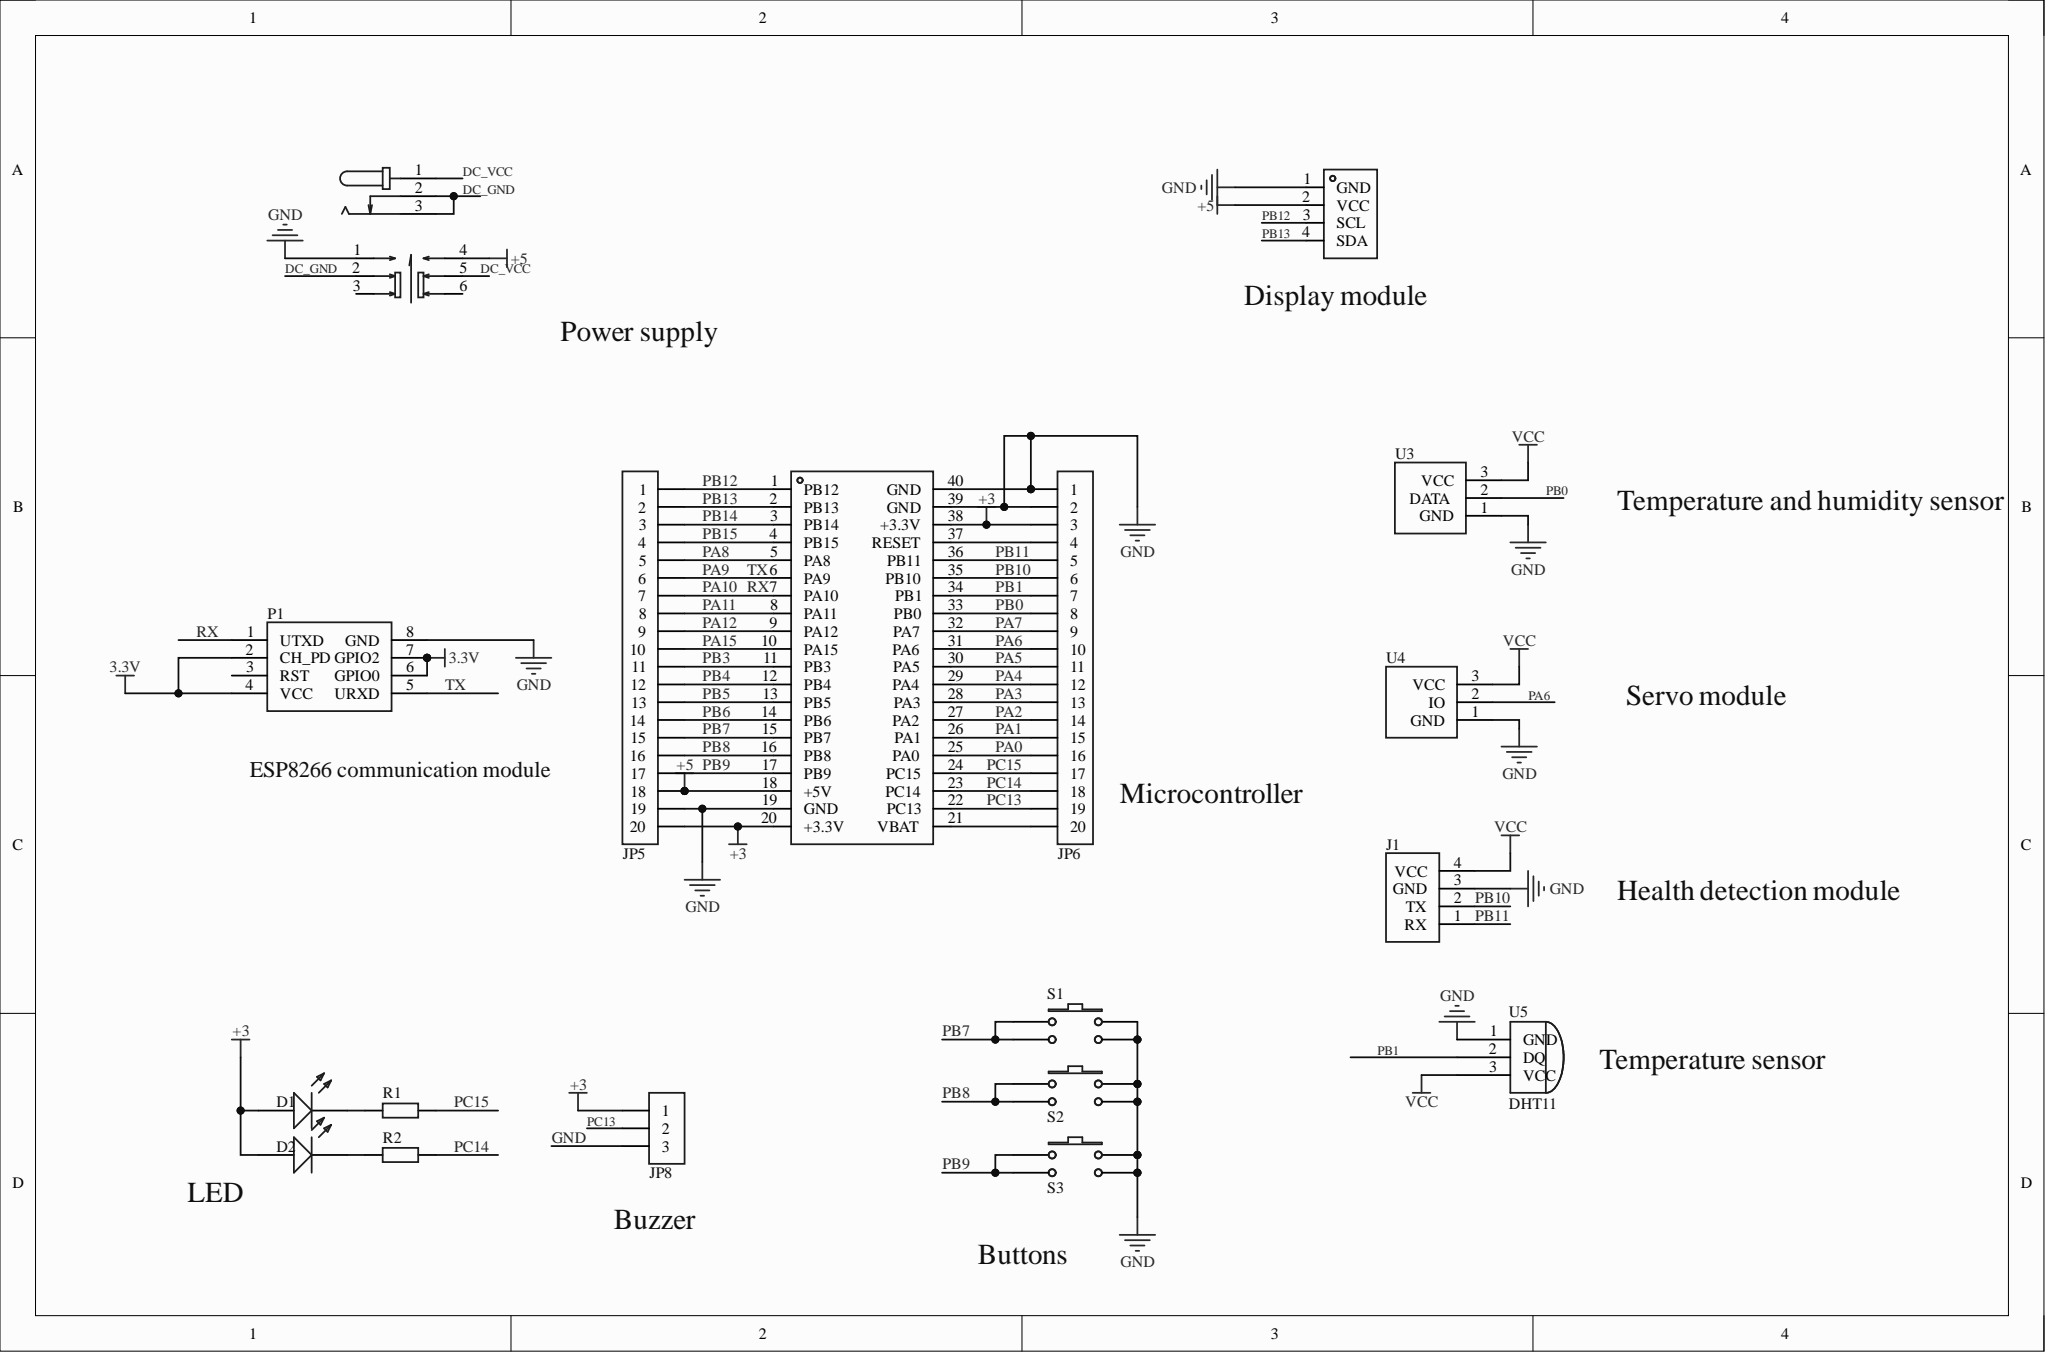Circuit board | Altium Designer | 19 parts | 43 nets
Bill of materials:
Comment,Description,Designator,Footprint,LibRef,Quantity
"led","","D1, D2","LED-TH_5mm","led","2"
"DC002-1.3","","DC1","DC-IN-TH_DC002-1.3","DC002-1.3","1"
"","Header, 4-Pin","J1","HDR-TH_4P-P2.54-V-F","J1","1"
"HDR-1X20","20P connector","JP5","HDR-TH_20P-P2.54-V-F","HDR-1X20","1"
"HDR-1X20","20P connector","JP6","HDR-TH_20P-P2.54-V-F-6","HDR-1X20","1"
"HDR-1X3","3P connector","JP8","HDR-TH_3P-P2.54-V-F-4","HDR-1X3","1"
"","Header, 5-Pin, Dual row","P1","ESP8266-1","P1","1"
"Res2","Resistor","R1, R2","Res_1/8W","Res2","2"
"key_4","","S1, S2, S3","SW-TH_4P-L6.0-W6.0-P4.50-LS6.5","key_4","3"
"Self-lock button","","SW1","SW-TH_6P-L7.0-W7.0-P2.00","自锁按键","1"
"OLED","","U1","OLED-TH_L27.8-W27.2-P2.54_C9900033791","OLED","1"
"ST32F103C8T6","","U2","CONN-TH_L53.3-W22.9_STM32F103C8T6-CARD","ST32F103C8T6","1"
"","Programmable digital thermometer","U3, U4","HDR-TH_3P-P2.54-V-F","U3, U4","2"
"DHT11","","U5","HDR-TH_3P-P2.54-V-F","DHT11","1"
Netlist (Protel format):
[
D1
LED-TH_5mm
led



]
[
D2
LED-TH_5mm
led



]
[
DC1
DC-IN-TH_DC002-1.3
DC002-1.3



]
[
J1
HDR-TH_4P-P2.54-V-F




]
[
JP5
HDR-TH_20P-P2.54-V-F
HDR-1X20



]
[
JP6
HDR-TH_20P-P2.54-V-F-6
HDR-1X20



]
[
JP8
HDR-TH_3P-P2.54-V-F-4
HDR-1X3



]
[
P1
ESP8266-1




]
[
R1
Res_1/8W
Res2



]
[
R2
Res_1/8W
Res2



]
[
S1
SW-TH_4P-L6.0-W6.0-P4.50-LS6.5
key_4



]
[
S2
SW-TH_4P-L6.0-W6.0-P4.50-LS6.5
key_4



]
[
S3
SW-TH_4P-L6.0-W6.0-P4.50-LS6.5
key_4



]
[
SW1
SW-TH_6P-L7.0-W7.0-P2.00
Self-lock button



]
[
U1
OLED-TH_L27.8-W27.2-P2.54_C9900033791
OLED



]
[
U2
CONN-TH_L53.3-W22.9_STM32F103C8T6-CARD
ST32F103C8T6



]
[
U3
HDR-TH_3P-P2.54-V-F




]
[
U4
HDR-TH_3P-P2.54-V-F




]
[
U5
HDR-TH_3P-P2.54-V-F
DHT11



]
(
VCC
J1-4
U3-3
U4-3
U5-3
)
(
PC15
JP6-17
R1-2
U2-24
)
(
PC14
JP6-18
R2-2
U2-23
)
(
PC13
JP6-19
JP8-2
U2-22
)
(
PB15
JP5-4
U2-4
)
(
PB14
JP5-3
U2-3
)
(
PB13
JP5-2
U1-4
U2-2
)
(
PB12
JP5-1
U1-3
U2-1
)
(
PB11
J1-1
JP6-5
U2-36
)
(
PB10
J1-2
JP6-6
U2-35
)
(
PB9
JP5-17
S3-1
S3-3
U2-17
)
(
PB8
JP5-16
S2-1
S2-3
U2-16
)
(
PB7
JP5-15
S1-1
S1-3
U2-15
)
(
PB6
JP5-14
U2-14
)
(
PB5
JP5-13
U2-13
)
(
PB4
JP5-12
U2-12
)
(
PB3
JP5-11
U2-11
)
(
PB1
JP6-7
U2-34
U5-2
)
(
PB0
JP6-8
U2-33
U3-2
)
(
PA15
JP5-10
U2-10
)
(
PA12
JP5-9
U2-9
)
(
PA11
JP5-8
U2-8
)
(
PA10
JP5-7
P1-1
U2-7
)
(
PA9
JP5-6
P1-5
U2-6
)
(
PA8
JP5-5
U2-5
)
(
PA7
JP6-9
U2-32
)
(
PA6
JP6-10
U2-31
U4-2
)
(
PA5
JP6-11
U2-30
)
(
PA4
JP6-12
U2-29
)
(
PA3
JP6-13
U2-28
)
(
PA2
JP6-14
U2-27
)
(
PA1
JP6-15
U2-26
)
(
PA0
JP6-16
U2-25
)
(
NetJP6_20
JP6-20
U2-21
)
(
NetJP6_4
JP6-4
U2-37
)
(
NetD2_2
D2-2
R2-1
)
(
NetD1_2
D1-2
R1-1
)
(
GND
J1-3
JP5-19
JP6-1
JP6-2
JP8-3
P1-8
S1-2
S1-4
S2-2
S2-4
S3-2
S3-4
SW1-1
U1-1
U2-19
U2-39
U2-40
U3-1
U4-1
U5-1
)
(
DC_VCC
DC1-1
SW1-5
)
(
DC_GND
DC1-2
DC1-3
SW1-2
)
(
+5
JP5-18
SW1-4
U1-2
U2-18
)
(
+3
D1-1
D2-1
JP5-20
JP6-3
JP8-1
U2-20
U2-38
)
(
3.3V
P1-2
P1-4
P1-6
P1-7
)